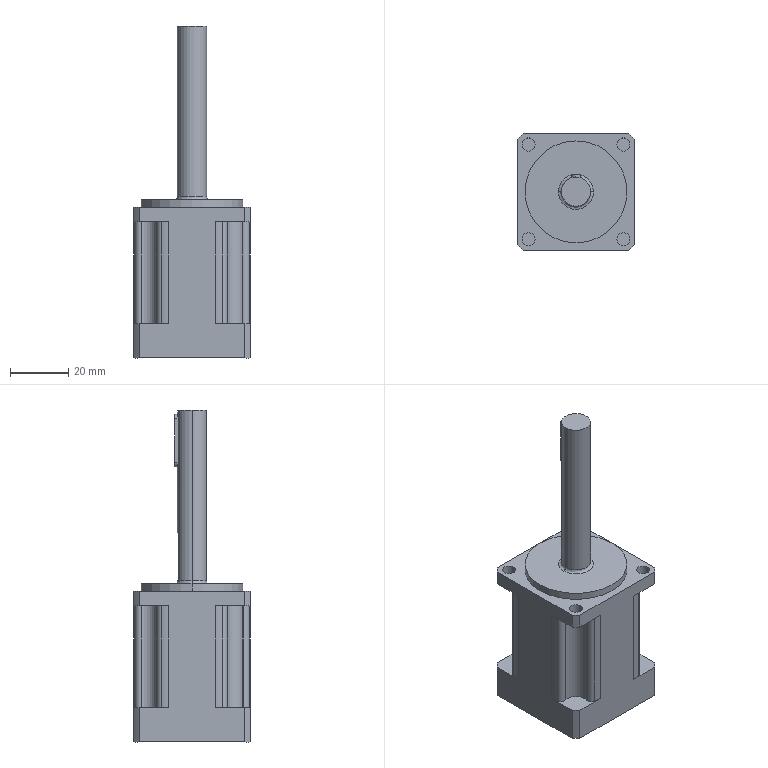Part | SolidWorks | features ICE 5, BaseBody 1 | 1 solid | 74 faces | box 40 x 40 x 114 mm | volume 76239 mm3 | cylinder 51 | plane 21 | spline 2 | commonest cylinder face diameters 4 x10 4.5 x8 24 x8 54 x8 8.5 x6 10 x4